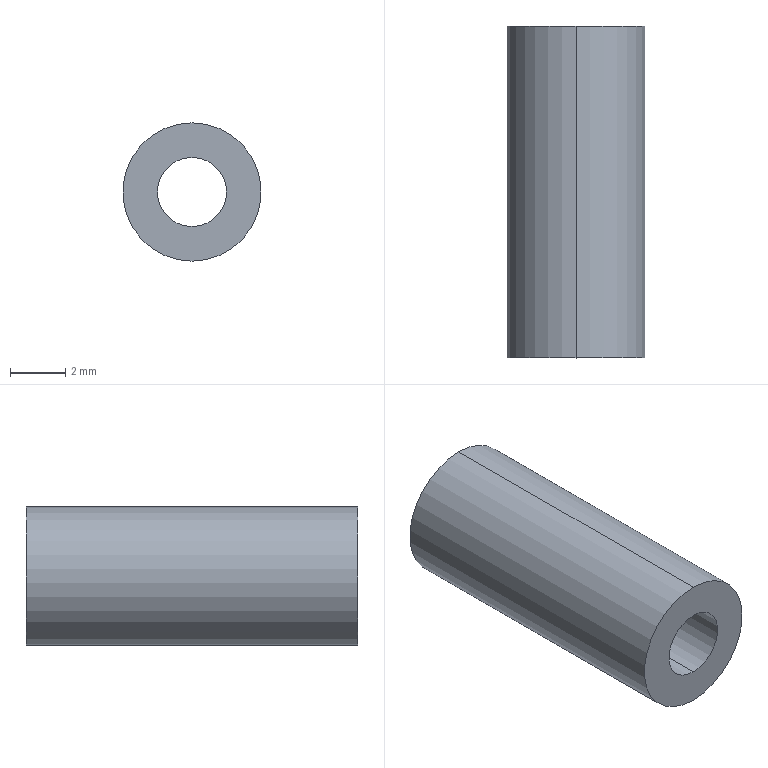Part | SolidWorks | features Extrusion 1, HoleWzd 1 | 1 solid | 6 faces | box 5 x 12 x 5 mm | volume 176.715 mm3 | cylinder 4 | plane 2 | commonest cylinder face diameters 2.5 x2 5 x2
STEP:
#1=CARTESIAN_POINT('',(0.,0.,-1.25));
#2=VERTEX_POINT('',#1);
#3=CARTESIAN_POINT('',(0.,0.,1.25));
#4=VERTEX_POINT('',#3);
#5=CARTESIAN_POINT('',(0.,0.,0.));
#6=DIRECTION('',(0.,1.,0.));
#7=DIRECTION('',(0.,0.,1.));
#8=AXIS2_PLACEMENT_3D('',#5,#6,#7);
#9=CIRCLE('',#8,1.25);
#10=EDGE_CURVE('',#2,#4,#9,.T.);
#11=ORIENTED_EDGE('',*,*,#10,.F.);
#12=CARTESIAN_POINT('',(0.,12.,-1.25));
#13=VERTEX_POINT('',#12);
#14=CARTESIAN_POINT('',(0.,12.,-1.25));
#15=DIRECTION('',(0.,1.,0.));
#16=VECTOR('',#15,1000.);
#17=LINE('',#14,#16);
#18=EDGE_CURVE('',#2,#13,#17,.T.);
#19=ORIENTED_EDGE('',*,*,#18,.T.);
#20=CARTESIAN_POINT('',(0.,12.,1.25));
#21=VERTEX_POINT('',#20);
#22=CARTESIAN_POINT('',(0.,12.,0.));
#23=DIRECTION('',(0.,1.,0.));
#24=DIRECTION('',(0.,0.,1.));
#25=AXIS2_PLACEMENT_3D('',#22,#23,#24);
#26=CIRCLE('',#25,1.25);
#27=EDGE_CURVE('',#13,#21,#26,.T.);
#28=ORIENTED_EDGE('',*,*,#27,.T.);
#29=CARTESIAN_POINT('',(0.,12.,1.25));
#30=DIRECTION('',(0.,1.,0.));
#31=VECTOR('',#30,1000.);
#32=LINE('',#29,#31);
#33=EDGE_CURVE('',#4,#21,#32,.T.);
#34=ORIENTED_EDGE('',*,*,#33,.F.);
#35=EDGE_LOOP('',(#11,#19,#28,#34));
#36=FACE_OUTER_BOUND('',#35,.T.);
#37=CARTESIAN_POINT('',(0.,12.,0.));
#38=DIRECTION('',(0.,1.,0.));
#39=DIRECTION('',(0.,0.,1.));
#40=AXIS2_PLACEMENT_3D('',#37,#38,#39);
#41=CYLINDRICAL_SURFACE('',#40,1.25);
#42=ADVANCED_FACE('',(#36),#41,.F.);
#43=CARTESIAN_POINT('',(0.,12.,2.5));
#44=VERTEX_POINT('',#43);
#45=CARTESIAN_POINT('',(0.,12.,-2.5));
#46=VERTEX_POINT('',#45);
#47=CARTESIAN_POINT('',(0.,12.,0.));
#48=DIRECTION('',(0.,1.,0.));
#49=DIRECTION('',(0.,0.,1.));
#50=AXIS2_PLACEMENT_3D('',#47,#48,#49);
#51=CIRCLE('',#50,2.5);
#52=EDGE_CURVE('',#44,#46,#51,.T.);
#53=ORIENTED_EDGE('',*,*,#52,.F.);
#54=CARTESIAN_POINT('',(0.,0.,2.5));
#55=VERTEX_POINT('',#54);
#56=CARTESIAN_POINT('',(0.,12.,2.5));
#57=DIRECTION('',(0.,-1.,0.));
#58=VECTOR('',#57,1000.);
#59=LINE('',#56,#58);
#60=EDGE_CURVE('',#44,#55,#59,.T.);
#61=ORIENTED_EDGE('',*,*,#60,.T.);
#62=CARTESIAN_POINT('',(0.,0.,-2.5));
#63=VERTEX_POINT('',#62);
#64=CARTESIAN_POINT('',(0.,0.,0.));
#65=DIRECTION('',(0.,1.,0.));
#66=DIRECTION('',(0.,0.,1.));
#67=AXIS2_PLACEMENT_3D('',#64,#65,#66);
#68=CIRCLE('',#67,2.5);
#69=EDGE_CURVE('',#55,#63,#68,.T.);
#70=ORIENTED_EDGE('',*,*,#69,.T.);
#71=CARTESIAN_POINT('',(0.,12.,-2.5));
#72=DIRECTION('',(0.,-1.,0.));
#73=VECTOR('',#72,1000.);
#74=LINE('',#71,#73);
#75=EDGE_CURVE('',#46,#63,#74,.T.);
#76=ORIENTED_EDGE('',*,*,#75,.F.);
#77=EDGE_LOOP('',(#53,#61,#70,#76));
#78=FACE_OUTER_BOUND('',#77,.T.);
#79=CARTESIAN_POINT('',(0.,12.,0.));
#80=DIRECTION('',(0.,-1.,0.));
#81=DIRECTION('',(0.,0.,-1.));
#82=AXIS2_PLACEMENT_3D('',#79,#80,#81);
#83=CYLINDRICAL_SURFACE('',#82,2.5);
#84=ADVANCED_FACE('',(#78),#83,.T.);
#85=ORIENTED_EDGE('',*,*,#60,.F.);
#86=CARTESIAN_POINT('',(0.,12.,0.));
#87=DIRECTION('',(0.,1.,0.));
#88=DIRECTION('',(0.,0.,1.));
#89=AXIS2_PLACEMENT_3D('',#86,#87,#88);
#90=CIRCLE('',#89,2.5);
#91=EDGE_CURVE('',#46,#44,#90,.T.);
#92=ORIENTED_EDGE('',*,*,#91,.F.);
#93=ORIENTED_EDGE('',*,*,#75,.T.);
#94=CARTESIAN_POINT('',(0.,0.,0.));
#95=DIRECTION('',(0.,1.,0.));
#96=DIRECTION('',(0.,0.,1.));
#97=AXIS2_PLACEMENT_3D('',#94,#95,#96);
#98=CIRCLE('',#97,2.5);
#99=EDGE_CURVE('',#63,#55,#98,.T.);
#100=ORIENTED_EDGE('',*,*,#99,.T.);
#101=EDGE_LOOP('',(#85,#92,#93,#100));
#102=FACE_OUTER_BOUND('',#101,.T.);
#103=CARTESIAN_POINT('',(0.,12.,0.));
#104=DIRECTION('',(0.,-1.,0.));
#105=DIRECTION('',(0.,0.,-1.));
#106=AXIS2_PLACEMENT_3D('',#103,#104,#105);
#107=CYLINDRICAL_SURFACE('',#106,2.5);
#108=ADVANCED_FACE('',(#102),#107,.T.);
#109=CARTESIAN_POINT('',(0.,12.,0.));
#110=DIRECTION('',(0.,1.,0.));
#111=DIRECTION('',(0.,0.,1.));
#112=AXIS2_PLACEMENT_3D('',#109,#110,#111);
#113=CIRCLE('',#112,1.25);
#114=EDGE_CURVE('',#21,#13,#113,.T.);
#115=ORIENTED_EDGE('',*,*,#114,.F.);
#116=ORIENTED_EDGE('',*,*,#27,.F.);
#117=EDGE_LOOP('',(#115,#116));
#118=FACE_BOUND('',#117,.T.);
#119=ORIENTED_EDGE('',*,*,#91,.T.);
#120=ORIENTED_EDGE('',*,*,#52,.T.);
#121=EDGE_LOOP('',(#119,#120));
#122=FACE_OUTER_BOUND('',#121,.T.);
#123=CARTESIAN_POINT('',(0.,12.,0.));
#124=DIRECTION('',(0.,1.,0.));
#125=DIRECTION('',(0.,0.,1.));
#126=AXIS2_PLACEMENT_3D('',#123,#124,#125);
#127=PLANE('',#126);
#128=ADVANCED_FACE('',(#118,#122),#127,.T.);
#129=CARTESIAN_POINT('',(0.,0.,0.));
#130=DIRECTION('',(0.,1.,0.));
#131=DIRECTION('',(0.,0.,1.));
#132=AXIS2_PLACEMENT_3D('',#129,#130,#131);
#133=CIRCLE('',#132,1.25);
#134=EDGE_CURVE('',#4,#2,#133,.T.);
#135=ORIENTED_EDGE('',*,*,#134,.T.);
#136=ORIENTED_EDGE('',*,*,#10,.T.);
#137=EDGE_LOOP('',(#135,#136));
#138=FACE_BOUND('',#137,.T.);
#139=ORIENTED_EDGE('',*,*,#99,.F.);
#140=ORIENTED_EDGE('',*,*,#69,.F.);
#141=EDGE_LOOP('',(#139,#140));
#142=FACE_OUTER_BOUND('',#141,.T.);
#143=CARTESIAN_POINT('',(0.,0.,0.));
#144=DIRECTION('',(0.,1.,0.));
#145=DIRECTION('',(0.,0.,1.));
#146=AXIS2_PLACEMENT_3D('',#143,#144,#145);
#147=PLANE('',#146);
#148=ADVANCED_FACE('',(#138,#142),#147,.F.);
#149=ORIENTED_EDGE('',*,*,#18,.F.);
#150=ORIENTED_EDGE('',*,*,#134,.F.);
#151=ORIENTED_EDGE('',*,*,#33,.T.);
#152=ORIENTED_EDGE('',*,*,#114,.T.);
#153=EDGE_LOOP('',(#149,#150,#151,#152));
#154=FACE_OUTER_BOUND('',#153,.T.);
#155=CARTESIAN_POINT('',(0.,12.,0.));
#156=DIRECTION('',(0.,1.,0.));
#157=DIRECTION('',(0.,0.,1.));
#158=AXIS2_PLACEMENT_3D('',#155,#156,#157);
#159=CYLINDRICAL_SURFACE('',#158,1.25);
#160=ADVANCED_FACE('',(#154),#159,.F.);
#161=CLOSED_SHELL('',(#42,#84,#108,#128,#148,#160));
#162=MANIFOLD_SOLID_BREP('',#161);
#163=CARTESIAN_POINT('',(0.,0.,0.));
#164=DIRECTION('',(0.,0.,1.));
#165=DIRECTION('',(1.,0.,0.));
#166=AXIS2_PLACEMENT_3D('',#163,#164,#165);
#167=(LENGTH_UNIT()NAMED_UNIT(*)SI_UNIT(.MILLI.,.METRE.));
#168=UNCERTAINTY_MEASURE_WITH_UNIT(LENGTH_MEASURE(0.00001),#167,'','');
#169=(NAMED_UNIT(*)PLANE_ANGLE_UNIT()SI_UNIT($,.RADIAN.));
#170=(NAMED_UNIT(*)SI_UNIT($,.STERADIAN.)SOLID_ANGLE_UNIT());
#171=(GEOMETRIC_REPRESENTATION_CONTEXT(3)GLOBAL_UNCERTAINTY_ASSIGNED_CONTEXT((#168))GLOBAL_UNIT_ASSIGNED_CONTEXT((#167,#169,#170))REPRESENTATION_CONTEXT('',''));
#172=ADVANCED_BREP_SHAPE_REPRESENTATION('',(#162,#166),#171);